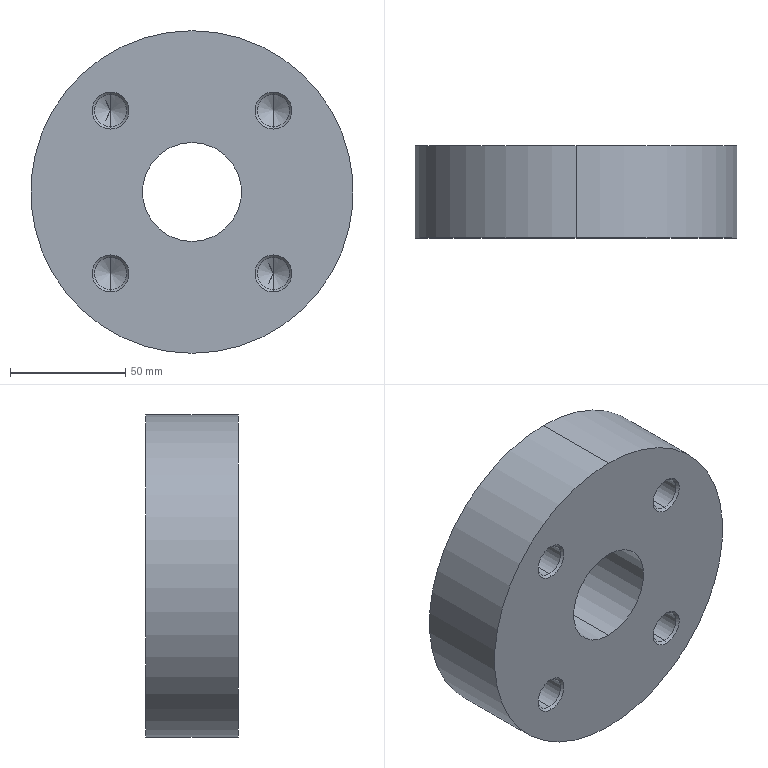Part | SolidWorks | features HoleWzd 2, Extrusion 1 | 1 solid | 54 faces | box 140 x 40 x 140 mm | volume 521515 mm3 | cone 32 | cylinder 20 | plane 2 | commonest cylinder face diameters 14 x16 43 x2 140 x2
STEP:
#1=CARTESIAN_POINT('',(35.355,1.025,-28.355));
#2=VERTEX_POINT('',#1);
#3=CARTESIAN_POINT('',(35.355,1.025,-42.355));
#4=VERTEX_POINT('',#3);
#5=CARTESIAN_POINT('',(35.355,1.025,-35.355));
#6=DIRECTION('',(0.,-1.,0.));
#7=DIRECTION('',(0.,0.,-1.));
#8=AXIS2_PLACEMENT_3D('',#5,#6,#7);
#9=CIRCLE('',#8,7.);
#10=EDGE_CURVE('',#2,#4,#9,.T.);
#11=ORIENTED_EDGE('',*,*,#10,.F.);
#12=CARTESIAN_POINT('',(35.355,0.,-27.33));
#13=VERTEX_POINT('',#12);
#14=CARTESIAN_POINT('',(35.355,0.,-27.33));
#15=DIRECTION('',(0.,-0.7071,0.7071));
#16=VECTOR('',#15,1000.);
#17=LINE('',#14,#16);
#18=EDGE_CURVE('',#2,#13,#17,.T.);
#19=ORIENTED_EDGE('',*,*,#18,.T.);
#20=CARTESIAN_POINT('',(35.355,0.,-43.38));
#21=VERTEX_POINT('',#20);
#22=CARTESIAN_POINT('',(35.355,0.,-35.355));
#23=DIRECTION('',(0.,-1.,0.));
#24=DIRECTION('',(0.,0.,-1.));
#25=AXIS2_PLACEMENT_3D('',#22,#23,#24);
#26=CIRCLE('',#25,8.025);
#27=EDGE_CURVE('',#13,#21,#26,.T.);
#28=ORIENTED_EDGE('',*,*,#27,.T.);
#29=CARTESIAN_POINT('',(35.355,0.,-43.38));
#30=DIRECTION('',(0.,-0.7071,-0.7071));
#31=VECTOR('',#30,1000.);
#32=LINE('',#29,#31);
#33=EDGE_CURVE('',#4,#21,#32,.T.);
#34=ORIENTED_EDGE('',*,*,#33,.F.);
#35=EDGE_LOOP('',(#11,#19,#28,#34));
#36=FACE_OUTER_BOUND('',#35,.T.);
#37=CARTESIAN_POINT('',(35.355,0.,-35.355));
#38=DIRECTION('',(0.,-1.,0.));
#39=DIRECTION('',(0.,0.,-1.));
#40=AXIS2_PLACEMENT_3D('',#37,#38,#39);
#41=CONICAL_SURFACE('',#40,8.025,0.7854);
#42=ADVANCED_FACE('',(#36),#41,.F.);
#43=CARTESIAN_POINT('',(35.355,27.794,-28.355));
#44=VERTEX_POINT('',#43);
#45=CARTESIAN_POINT('',(35.355,27.794,-42.355));
#46=VERTEX_POINT('',#45);
#47=CARTESIAN_POINT('',(35.355,27.794,-35.355));
#48=DIRECTION('',(0.,-1.,0.));
#49=DIRECTION('',(0.,0.,-1.));
#50=AXIS2_PLACEMENT_3D('',#47,#48,#49);
#51=CIRCLE('',#50,7.);
#52=EDGE_CURVE('',#44,#46,#51,.T.);
#53=ORIENTED_EDGE('',*,*,#52,.F.);
#54=CARTESIAN_POINT('',(35.355,0.,-28.355));
#55=DIRECTION('',(0.,-1.,0.));
#56=VECTOR('',#55,1000.);
#57=LINE('',#54,#56);
#58=EDGE_CURVE('',#44,#2,#57,.T.);
#59=ORIENTED_EDGE('',*,*,#58,.T.);
#60=ORIENTED_EDGE('',*,*,#10,.T.);
#61=CARTESIAN_POINT('',(35.355,0.,-42.355));
#62=DIRECTION('',(0.,-1.,0.));
#63=VECTOR('',#62,1000.);
#64=LINE('',#61,#63);
#65=EDGE_CURVE('',#46,#4,#64,.T.);
#66=ORIENTED_EDGE('',*,*,#65,.F.);
#67=EDGE_LOOP('',(#53,#59,#60,#66));
#68=FACE_OUTER_BOUND('',#67,.T.);
#69=CARTESIAN_POINT('',(35.355,0.,-35.355));
#70=DIRECTION('',(0.,-1.,0.));
#71=DIRECTION('',(0.,0.,-1.));
#72=AXIS2_PLACEMENT_3D('',#69,#70,#71);
#73=CYLINDRICAL_SURFACE('',#72,7.);
#74=ADVANCED_FACE('',(#68),#73,.F.);
#75=CARTESIAN_POINT('',(35.355,32.,-35.355));
#76=VERTEX_POINT('',#75);
#77=CARTESIAN_POINT('',(35.355,27.794,-42.355));
#78=DIRECTION('',(0.,-0.515,-0.8572));
#79=VECTOR('',#78,1000.);
#80=LINE('',#77,#79);
#81=EDGE_CURVE('',#76,#46,#80,.T.);
#82=ORIENTED_EDGE('',*,*,#81,.F.);
#83=CARTESIAN_POINT('',(35.355,27.794,-28.355));
#84=DIRECTION('',(0.,-0.515,0.8572));
#85=VECTOR('',#84,1000.);
#86=LINE('',#83,#85);
#87=EDGE_CURVE('',#76,#44,#86,.T.);
#88=ORIENTED_EDGE('',*,*,#87,.T.);
#89=ORIENTED_EDGE('',*,*,#52,.T.);
#90=EDGE_LOOP('',(#82,#88,#89));
#91=FACE_OUTER_BOUND('',#90,.T.);
#92=CARTESIAN_POINT('',(35.355,27.794,-35.355));
#93=DIRECTION('',(0.,-1.,0.));
#94=DIRECTION('',(0.,0.,-1.));
#95=AXIS2_PLACEMENT_3D('',#92,#93,#94);
#96=CONICAL_SURFACE('',#95,7.,1.03);
#97=ADVANCED_FACE('',(#91),#96,.F.);
#98=CARTESIAN_POINT('',(-35.355,1.025,-28.355));
#99=VERTEX_POINT('',#98);
#100=CARTESIAN_POINT('',(-35.355,1.025,-42.355));
#101=VERTEX_POINT('',#100);
#102=CARTESIAN_POINT('',(-35.355,1.025,-35.355));
#103=DIRECTION('',(0.,-1.,0.));
#104=DIRECTION('',(0.,0.,-1.));
#105=AXIS2_PLACEMENT_3D('',#102,#103,#104);
#106=CIRCLE('',#105,7.);
#107=EDGE_CURVE('',#99,#101,#106,.T.);
#108=ORIENTED_EDGE('',*,*,#107,.F.);
#109=CARTESIAN_POINT('',(-35.355,0.,-27.33));
#110=VERTEX_POINT('',#109);
#111=CARTESIAN_POINT('',(-35.355,0.,-27.33));
#112=DIRECTION('',(0.,-0.7071,0.7071));
#113=VECTOR('',#112,1000.);
#114=LINE('',#111,#113);
#115=EDGE_CURVE('',#99,#110,#114,.T.);
#116=ORIENTED_EDGE('',*,*,#115,.T.);
#117=CARTESIAN_POINT('',(-35.355,0.,-43.38));
#118=VERTEX_POINT('',#117);
#119=CARTESIAN_POINT('',(-35.355,0.,-35.355));
#120=DIRECTION('',(0.,-1.,0.));
#121=DIRECTION('',(0.,0.,-1.));
#122=AXIS2_PLACEMENT_3D('',#119,#120,#121);
#123=CIRCLE('',#122,8.025);
#124=EDGE_CURVE('',#110,#118,#123,.T.);
#125=ORIENTED_EDGE('',*,*,#124,.T.);
#126=CARTESIAN_POINT('',(-35.355,0.,-43.38));
#127=DIRECTION('',(0.,-0.7071,-0.7071));
#128=VECTOR('',#127,1000.);
#129=LINE('',#126,#128);
#130=EDGE_CURVE('',#101,#118,#129,.T.);
#131=ORIENTED_EDGE('',*,*,#130,.F.);
#132=EDGE_LOOP('',(#108,#116,#125,#131));
#133=FACE_OUTER_BOUND('',#132,.T.);
#134=CARTESIAN_POINT('',(-35.355,0.,-35.355));
#135=DIRECTION('',(0.,-1.,0.));
#136=DIRECTION('',(0.,0.,-1.));
#137=AXIS2_PLACEMENT_3D('',#134,#135,#136);
#138=CONICAL_SURFACE('',#137,8.025,0.7854);
#139=ADVANCED_FACE('',(#133),#138,.F.);
#140=CARTESIAN_POINT('',(-35.355,27.794,-28.355));
#141=VERTEX_POINT('',#140);
#142=CARTESIAN_POINT('',(-35.355,27.794,-42.355));
#143=VERTEX_POINT('',#142);
#144=CARTESIAN_POINT('',(-35.355,27.794,-35.355));
#145=DIRECTION('',(0.,-1.,0.));
#146=DIRECTION('',(0.,0.,-1.));
#147=AXIS2_PLACEMENT_3D('',#144,#145,#146);
#148=CIRCLE('',#147,7.);
#149=EDGE_CURVE('',#141,#143,#148,.T.);
#150=ORIENTED_EDGE('',*,*,#149,.F.);
#151=CARTESIAN_POINT('',(-35.355,0.,-28.355));
#152=DIRECTION('',(0.,-1.,0.));
#153=VECTOR('',#152,1000.);
#154=LINE('',#151,#153);
#155=EDGE_CURVE('',#141,#99,#154,.T.);
#156=ORIENTED_EDGE('',*,*,#155,.T.);
#157=ORIENTED_EDGE('',*,*,#107,.T.);
#158=CARTESIAN_POINT('',(-35.355,0.,-42.355));
#159=DIRECTION('',(0.,-1.,0.));
#160=VECTOR('',#159,1000.);
#161=LINE('',#158,#160);
#162=EDGE_CURVE('',#143,#101,#161,.T.);
#163=ORIENTED_EDGE('',*,*,#162,.F.);
#164=EDGE_LOOP('',(#150,#156,#157,#163));
#165=FACE_OUTER_BOUND('',#164,.T.);
#166=CARTESIAN_POINT('',(-35.355,0.,-35.355));
#167=DIRECTION('',(0.,-1.,0.));
#168=DIRECTION('',(0.,0.,-1.));
#169=AXIS2_PLACEMENT_3D('',#166,#167,#168);
#170=CYLINDRICAL_SURFACE('',#169,7.);
#171=ADVANCED_FACE('',(#165),#170,.F.);
#172=CARTESIAN_POINT('',(-35.355,32.,-35.355));
#173=VERTEX_POINT('',#172);
#174=CARTESIAN_POINT('',(-35.355,27.794,-42.355));
#175=DIRECTION('',(0.,-0.515,-0.8572));
#176=VECTOR('',#175,1000.);
#177=LINE('',#174,#176);
#178=EDGE_CURVE('',#173,#143,#177,.T.);
#179=ORIENTED_EDGE('',*,*,#178,.F.);
#180=CARTESIAN_POINT('',(-35.355,27.794,-28.355));
#181=DIRECTION('',(0.,-0.515,0.8572));
#182=VECTOR('',#181,1000.);
#183=LINE('',#180,#182);
#184=EDGE_CURVE('',#173,#141,#183,.T.);
#185=ORIENTED_EDGE('',*,*,#184,.T.);
#186=ORIENTED_EDGE('',*,*,#149,.T.);
#187=EDGE_LOOP('',(#179,#185,#186));
#188=FACE_OUTER_BOUND('',#187,.T.);
#189=CARTESIAN_POINT('',(-35.355,27.794,-35.355));
#190=DIRECTION('',(0.,-1.,0.));
#191=DIRECTION('',(0.,0.,-1.));
#192=AXIS2_PLACEMENT_3D('',#189,#190,#191);
#193=CONICAL_SURFACE('',#192,7.,1.03);
#194=ADVANCED_FACE('',(#188),#193,.F.);
#195=CARTESIAN_POINT('',(-35.355,1.025,42.355));
#196=VERTEX_POINT('',#195);
#197=CARTESIAN_POINT('',(-35.355,1.025,28.355));
#198=VERTEX_POINT('',#197);
#199=CARTESIAN_POINT('',(-35.355,1.025,35.355));
#200=DIRECTION('',(0.,-1.,0.));
#201=DIRECTION('',(0.,0.,-1.));
#202=AXIS2_PLACEMENT_3D('',#199,#200,#201);
#203=CIRCLE('',#202,7.);
#204=EDGE_CURVE('',#196,#198,#203,.T.);
#205=ORIENTED_EDGE('',*,*,#204,.F.);
#206=CARTESIAN_POINT('',(-35.355,0.,43.38));
#207=VERTEX_POINT('',#206);
#208=CARTESIAN_POINT('',(-35.355,0.,43.38));
#209=DIRECTION('',(0.,-0.7071,0.7071));
#210=VECTOR('',#209,1000.);
#211=LINE('',#208,#210);
#212=EDGE_CURVE('',#196,#207,#211,.T.);
#213=ORIENTED_EDGE('',*,*,#212,.T.);
#214=CARTESIAN_POINT('',(-35.355,0.,27.33));
#215=VERTEX_POINT('',#214);
#216=CARTESIAN_POINT('',(-35.355,0.,35.355));
#217=DIRECTION('',(0.,-1.,0.));
#218=DIRECTION('',(0.,0.,-1.));
#219=AXIS2_PLACEMENT_3D('',#216,#217,#218);
#220=CIRCLE('',#219,8.025);
#221=EDGE_CURVE('',#207,#215,#220,.T.);
#222=ORIENTED_EDGE('',*,*,#221,.T.);
#223=CARTESIAN_POINT('',(-35.355,0.,27.33));
#224=DIRECTION('',(0.,-0.7071,-0.7071));
#225=VECTOR('',#224,1000.);
#226=LINE('',#223,#225);
#227=EDGE_CURVE('',#198,#215,#226,.T.);
#228=ORIENTED_EDGE('',*,*,#227,.F.);
#229=EDGE_LOOP('',(#205,#213,#222,#228));
#230=FACE_OUTER_BOUND('',#229,.T.);
#231=CARTESIAN_POINT('',(-35.355,0.,35.355));
#232=DIRECTION('',(0.,-1.,0.));
#233=DIRECTION('',(0.,0.,-1.));
#234=AXIS2_PLACEMENT_3D('',#231,#232,#233);
#235=CONICAL_SURFACE('',#234,8.025,0.7854);
#236=ADVANCED_FACE('',(#230),#235,.F.);
#237=CARTESIAN_POINT('',(-35.355,27.794,42.355));
#238=VERTEX_POINT('',#237);
#239=CARTESIAN_POINT('',(-35.355,27.794,28.355));
#240=VERTEX_POINT('',#239);
#241=CARTESIAN_POINT('',(-35.355,27.794,35.355));
#242=DIRECTION('',(0.,-1.,0.));
#243=DIRECTION('',(0.,0.,-1.));
#244=AXIS2_PLACEMENT_3D('',#241,#242,#243);
#245=CIRCLE('',#244,7.);
#246=EDGE_CURVE('',#238,#240,#245,.T.);
#247=ORIENTED_EDGE('',*,*,#246,.F.);
#248=CARTESIAN_POINT('',(-35.355,0.,42.355));
#249=DIRECTION('',(0.,-1.,0.));
#250=VECTOR('',#249,1000.);
#251=LINE('',#248,#250);
#252=EDGE_CURVE('',#238,#196,#251,.T.);
#253=ORIENTED_EDGE('',*,*,#252,.T.);
#254=ORIENTED_EDGE('',*,*,#204,.T.);
#255=CARTESIAN_POINT('',(-35.355,0.,28.355));
#256=DIRECTION('',(0.,-1.,0.));
#257=VECTOR('',#256,1000.);
#258=LINE('',#255,#257);
#259=EDGE_CURVE('',#240,#198,#258,.T.);
#260=ORIENTED_EDGE('',*,*,#259,.F.);
#261=EDGE_LOOP('',(#247,#253,#254,#260));
#262=FACE_OUTER_BOUND('',#261,.T.);
#263=CARTESIAN_POINT('',(-35.355,0.,35.355));
#264=DIRECTION('',(0.,-1.,0.));
#265=DIRECTION('',(0.,0.,-1.));
#266=AXIS2_PLACEMENT_3D('',#263,#264,#265);
#267=CYLINDRICAL_SURFACE('',#266,7.);
#268=ADVANCED_FACE('',(#262),#267,.F.);
#269=CARTESIAN_POINT('',(-35.355,32.,35.355));
#270=VERTEX_POINT('',#269);
#271=CARTESIAN_POINT('',(-35.355,27.794,28.355));
#272=DIRECTION('',(0.,-0.515,-0.8572));
#273=VECTOR('',#272,1000.);
#274=LINE('',#271,#273);
#275=EDGE_CURVE('',#270,#240,#274,.T.);
#276=ORIENTED_EDGE('',*,*,#275,.F.);
#277=CARTESIAN_POINT('',(-35.355,27.794,42.355));
#278=DIRECTION('',(0.,-0.515,0.8572));
#279=VECTOR('',#278,1000.);
#280=LINE('',#277,#279);
#281=EDGE_CURVE('',#270,#238,#280,.T.);
#282=ORIENTED_EDGE('',*,*,#281,.T.);
#283=ORIENTED_EDGE('',*,*,#246,.T.);
#284=EDGE_LOOP('',(#276,#282,#283));
#285=FACE_OUTER_BOUND('',#284,.T.);
#286=CARTESIAN_POINT('',(-35.355,27.794,35.355));
#287=DIRECTION('',(0.,-1.,0.));
#288=DIRECTION('',(0.,0.,-1.));
#289=AXIS2_PLACEMENT_3D('',#286,#287,#288);
#290=CONICAL_SURFACE('',#289,7.,1.03);
#291=ADVANCED_FACE('',(#285),#290,.F.);
#292=CARTESIAN_POINT('',(35.355,1.025,42.355));
#293=VERTEX_POINT('',#292);
#294=CARTESIAN_POINT('',(35.355,1.025,28.355));
#295=VERTEX_POINT('',#294);
#296=CARTESIAN_POINT('',(35.355,1.025,35.355));
#297=DIRECTION('',(0.,-1.,0.));
#298=DIRECTION('',(0.,0.,-1.));
#299=AXIS2_PLACEMENT_3D('',#296,#297,#298);
#300=CIRCLE('',#299,7.);
#301=EDGE_CURVE('',#293,#295,#300,.T.);
#302=ORIENTED_EDGE('',*,*,#301,.F.);
#303=CARTESIAN_POINT('',(35.355,0.,43.38));
#304=VERTEX_POINT('',#303);
#305=CARTESIAN_POINT('',(35.355,0.,43.38));
#306=DIRECTION('',(0.,-0.7071,0.7071));
#307=VECTOR('',#306,1000.);
#308=LINE('',#305,#307);
#309=EDGE_CURVE('',#293,#304,#308,.T.);
#310=ORIENTED_EDGE('',*,*,#309,.T.);
#311=CARTESIAN_POINT('',(35.355,0.,27.33));
#312=VERTEX_POINT('',#311);
#313=CARTESIAN_POINT('',(35.355,0.,35.355));
#314=DIRECTION('',(0.,-1.,0.));
#315=DIRECTION('',(0.,0.,-1.));
#316=AXIS2_PLACEMENT_3D('',#313,#314,#315);
#317=CIRCLE('',#316,8.025);
#318=EDGE_CURVE('',#304,#312,#317,.T.);
#319=ORIENTED_EDGE('',*,*,#318,.T.);
#320=CARTESIAN_POINT('',(35.355,0.,27.33));
#321=DIRECTION('',(0.,-0.7071,-0.7071));
#322=VECTOR('',#321,1000.);
#323=LINE('',#320,#322);
#324=EDGE_CURVE('',#295,#312,#323,.T.);
#325=ORIENTED_EDGE('',*,*,#324,.F.);
#326=EDGE_LOOP('',(#302,#310,#319,#325));
#327=FACE_OUTER_BOUND('',#326,.T.);
#328=CARTESIAN_POINT('',(35.355,0.,35.355));
#329=DIRECTION('',(0.,-1.,0.));
#330=DIRECTION('',(0.,0.,-1.));
#331=AXIS2_PLACEMENT_3D('',#328,#329,#330);
#332=CONICAL_SURFACE('',#331,8.025,0.7854);
#333=ADVANCED_FACE('',(#327),#332,.F.);
#334=CARTESIAN_POINT('',(35.355,27.794,42.355));
#335=VERTEX_POINT('',#334);
#336=CARTESIAN_POINT('',(35.355,27.794,28.355));
#337=VERTEX_POINT('',#336);
#338=CARTESIAN_POINT('',(35.355,27.794,35.355));
#339=DIRECTION('',(0.,-1.,0.));
#340=DIRECTION('',(0.,0.,-1.));
#341=AXIS2_PLACEMENT_3D('',#338,#339,#340);
#342=CIRCLE('',#341,7.);
#343=EDGE_CURVE('',#335,#337,#342,.T.);
#344=ORIENTED_EDGE('',*,*,#343,.F.);
#345=CARTESIAN_POINT('',(35.355,0.,42.355));
#346=DIRECTION('',(0.,-1.,0.));
#347=VECTOR('',#346,1000.);
#348=LINE('',#345,#347);
#349=EDGE_CURVE('',#335,#293,#348,.T.);
#350=ORIENTED_EDGE('',*,*,#349,.T.);
#351=ORIENTED_EDGE('',*,*,#301,.T.);
#352=CARTESIAN_POINT('',(35.355,0.,28.355));
#353=DIRECTION('',(0.,-1.,0.));
#354=VECTOR('',#353,1000.);
#355=LINE('',#352,#354);
#356=EDGE_CURVE('',#337,#295,#355,.T.);
#357=ORIENTED_EDGE('',*,*,#356,.F.);
#358=EDGE_LOOP('',(#344,#350,#351,#357));
#359=FACE_OUTER_BOUND('',#358,.T.);
#360=CARTESIAN_POINT('',(35.355,0.,35.355));
#361=DIRECTION('',(0.,-1.,0.));
#362=DIRECTION('',(0.,0.,-1.));
#363=AXIS2_PLACEMENT_3D('',#360,#361,#362);
#364=CYLINDRICAL_SURFACE('',#363,7.);
#365=ADVANCED_FACE('',(#359),#364,.F.);
#366=CARTESIAN_POINT('',(35.355,32.,35.355));
#367=VERTEX_POINT('',#366);
#368=CARTESIAN_POINT('',(35.355,27.794,28.355));
#369=DIRECTION('',(0.,-0.515,-0.8572));
#370=VECTOR('',#369,1000.);
#371=LINE('',#368,#370);
#372=EDGE_CURVE('',#367,#337,#371,.T.);
#373=ORIENTED_EDGE('',*,*,#372,.F.);
#374=CARTESIAN_POINT('',(35.355,27.794,42.355));
#375=DIRECTION('',(0.,-0.515,0.8572));
#376=VECTOR('',#375,1000.);
#377=LINE('',#374,#376);
#378=EDGE_CURVE('',#367,#335,#377,.T.);
#379=ORIENTED_EDGE('',*,*,#378,.T.);
#380=ORIENTED_EDGE('',*,*,#343,.T.);
#381=EDGE_LOOP('',(#373,#379,#380));
#382=FACE_OUTER_BOUND('',#381,.T.);
#383=CARTESIAN_POINT('',(35.355,27.794,35.355));
#384=DIRECTION('',(0.,-1.,0.));
#385=DIRECTION('',(0.,0.,-1.));
#386=AXIS2_PLACEMENT_3D('',#383,#384,#385);
#387=CONICAL_SURFACE('',#386,7.,1.03);
#388=ADVANCED_FACE('',(#382),#387,.F.);
#389=CARTESIAN_POINT('',(0.,38.975,-57.));
#390=VERTEX_POINT('',#389);
#391=CARTESIAN_POINT('',(0.,38.975,-43.));
#392=VERTEX_POINT('',#391);
#393=CARTESIAN_POINT('',(0.,38.975,-50.));
#394=DIRECTION('',(0.,1.,0.));
#395=DIRECTION('',(0.,0.,1.));
#396=AXIS2_PLACEMENT_3D('',#393,#394,#395);
#397=CIRCLE('',#396,7.);
#398=EDGE_CURVE('',#390,#392,#397,.T.);
#399=ORIENTED_EDGE('',*,*,#398,.F.);
#400=CARTESIAN_POINT('',(0.,40.,-58.025));
#401=VERTEX_POINT('',#400);
#402=CARTESIAN_POINT('',(0.,40.,-58.025));
#403=DIRECTION('',(0.,0.7071,-0.7071));
#404=VECTOR('',#403,1000.);
#405=LINE('',#402,#404);
#406=EDGE_CURVE('',#390,#401,#405,.T.);
#407=ORIENTED_EDGE('',*,*,#406,.T.);
#408=CARTESIAN_POINT('',(0.,40.,-41.975));
#409=VERTEX_POINT('',#408);
#410=CARTESIAN_POINT('',(0.,40.,-50.));
#411=DIRECTION('',(0.,1.,0.));
#412=DIRECTION('',(0.,0.,1.));
#413=AXIS2_PLACEMENT_3D('',#410,#411,#412);
#414=CIRCLE('',#413,8.025);
#415=EDGE_CURVE('',#401,#409,#414,.T.);
#416=ORIENTED_EDGE('',*,*,#415,.T.);
#417=CARTESIAN_POINT('',(0.,40.,-41.975));
#418=DIRECTION('',(0.,0.7071,0.7071));
#419=VECTOR('',#418,1000.);
#420=LINE('',#417,#419);
#421=EDGE_CURVE('',#392,#409,#420,.T.);
#422=ORIENTED_EDGE('',*,*,#421,.F.);
#423=EDGE_LOOP('',(#399,#407,#416,#422));
#424=FACE_OUTER_BOUND('',#423,.T.);
#425=CARTESIAN_POINT('',(0.,40.,-50.));
#426=DIRECTION('',(0.,1.,0.));
#427=DIRECTION('',(0.,0.,1.));
#428=AXIS2_PLACEMENT_3D('',#425,#426,#427);
#429=CONICAL_SURFACE('',#428,8.025,0.7854);
#430=ADVANCED_FACE('',(#424),#429,.F.);
#431=CARTESIAN_POINT('',(0.,12.206,-57.));
#432=VERTEX_POINT('',#431);
#433=CARTESIAN_POINT('',(0.,12.206,-43.));
#434=VERTEX_POINT('',#433);
#435=CARTESIAN_POINT('',(0.,12.206,-50.));
#436=DIRECTION('',(0.,1.,0.));
#437=DIRECTION('',(0.,0.,1.));
#438=AXIS2_PLACEMENT_3D('',#435,#436,#437);
#439=CIRCLE('',#438,7.);
#440=EDGE_CURVE('',#432,#434,#439,.T.);
#441=ORIENTED_EDGE('',*,*,#440,.F.);
#442=CARTESIAN_POINT('',(0.,40.,-57.));
#443=DIRECTION('',(0.,1.,0.));
#444=VECTOR('',#443,1000.);
#445=LINE('',#442,#444);
#446=EDGE_CURVE('',#432,#390,#445,.T.);
#447=ORIENTED_EDGE('',*,*,#446,.T.);
#448=ORIENTED_EDGE('',*,*,#398,.T.);
#449=CARTESIAN_POINT('',(0.,40.,-43.));
#450=DIRECTION('',(0.,1.,0.));
#451=VECTOR('',#450,1000.);
#452=LINE('',#449,#451);
#453=EDGE_CURVE('',#434,#392,#452,.T.);
#454=ORIENTED_EDGE('',*,*,#453,.F.);
#455=EDGE_LOOP('',(#441,#447,#448,#454));
#456=FACE_OUTER_BOUND('',#455,.T.);
#457=CARTESIAN_POINT('',(0.,40.,-50.));
#458=DIRECTION('',(0.,1.,0.));
#459=DIRECTION('',(0.,0.,1.));
#460=AXIS2_PLACEMENT_3D('',#457,#458,#459);
#461=CYLINDRICAL_SURFACE('',#460,7.);
#462=ADVANCED_FACE('',(#456),#461,.F.);
#463=CARTESIAN_POINT('',(0.,8.,-50.));
#464=VERTEX_POINT('',#463);
#465=CARTESIAN_POINT('',(0.,12.206,-43.));
#466=DIRECTION('',(0.,0.515,0.8572));
#467=VECTOR('',#466,1000.);
#468=LINE('',#465,#467);
#469=EDGE_CURVE('',#464,#434,#468,.T.);
#470=ORIENTED_EDGE('',*,*,#469,.F.);
#471=CARTESIAN_POINT('',(0.,12.206,-57.));
#472=DIRECTION('',(0.,0.515,-0.8572));
#473=VECTOR('',#472,1000.);
#474=LINE('',#471,#473);
#475=EDGE_CURVE('',#464,#432,#474,.T.);
#476=ORIENTED_EDGE('',*,*,#475,.T.);
#477=ORIENTED_EDGE('',*,*,#440,.T.);
#478=EDGE_LOOP('',(#470,#476,#477));
#479=FACE_OUTER_BOUND('',#478,.T.);
#480=CARTESIAN_POINT('',(0.,12.206,-50.));
#481=DIRECTION('',(0.,1.,0.));
#482=DIRECTION('',(0.,0.,1.));
#483=AXIS2_PLACEMENT_3D('',#480,#481,#482);
#484=CONICAL_SURFACE('',#483,7.,1.03);
#485=ADVANCED_FACE('',(#479),#484,.F.);
#486=CARTESIAN_POINT('',(50.,38.975,-7.));
#487=VERTEX_POINT('',#486);
#488=CARTESIAN_POINT('',(50.,38.975,7.));
#489=VERTEX_POINT('',#488);
#490=CARTESIAN_POINT('',(50.,38.975,0.));
#491=DIRECTION('',(0.,1.,0.));
#492=DIRECTION('',(0.,0.,1.));
#493=AXIS2_PLACEMENT_3D('',#490,#491,#492);
#494=CIRCLE('',#493,7.);
#495=EDGE_CURVE('',#487,#489,#494,.T.);
#496=ORIENTED_EDGE('',*,*,#495,.F.);
#497=CARTESIAN_POINT('',(50.,40.,-8.025));
#498=VERTEX_POINT('',#497);
#499=CARTESIAN_POINT('',(50.,40.,-8.025));
#500=DIRECTION('',(0.,0.7071,-0.7071));
#501=VECTOR('',#500,1000.);
#502=LINE('',#499,#501);
#503=EDGE_CURVE('',#487,#498,#502,.T.);
#504=ORIENTED_EDGE('',*,*,#503,.T.);
#505=CARTESIAN_POINT('',(50.,40.,8.025));
#506=VERTEX_POINT('',#505);
#507=CARTESIAN_POINT('',(50.,40.,0.));
#508=DIRECTION('',(0.,1.,0.));
#509=DIRECTION('',(0.,0.,1.));
#510=AXIS2_PLACEMENT_3D('',#507,#508,#509);
#511=CIRCLE('',#510,8.025);
#512=EDGE_CURVE('',#498,#506,#511,.T.);
#513=ORIENTED_EDGE('',*,*,#512,.T.);
#514=CARTESIAN_POINT('',(50.,40.,8.025));
#515=DIRECTION('',(0.,0.7071,0.7071));
#516=VECTOR('',#515,1000.);
#517=LINE('',#514,#516);
#518=EDGE_CURVE('',#489,#506,#517,.T.);
#519=ORIENTED_EDGE('',*,*,#518,.F.);
#520=EDGE_LOOP('',(#496,#504,#513,#519));
#521=FACE_OUTER_BOUND('',#520,.T.);
#522=CARTESIAN_POINT('',(50.,40.,0.));
#523=DIRECTION('',(0.,1.,0.));
#524=DIRECTION('',(0.,0.,1.));
#525=AXIS2_PLACEMENT_3D('',#522,#523,#524);
#526=CONICAL_SURFACE('',#525,8.025,0.7854);
#527=ADVANCED_FACE('',(#521),#526,.F.);
#528=CARTESIAN_POINT('',(50.,12.206,-7.));
#529=VERTEX_POINT('',#528);
#530=CARTESIAN_POINT('',(50.,12.206,7.));
#531=VERTEX_POINT('',#530);
#532=CARTESIAN_POINT('',(50.,12.206,0.));
#533=DIRECTION('',(0.,1.,0.));
#534=DIRECTION('',(0.,0.,1.));
#535=AXIS2_PLACEMENT_3D('',#532,#533,#534);
#536=CIRCLE('',#535,7.);
#537=EDGE_CURVE('',#529,#531,#536,.T.);
#538=ORIENTED_EDGE('',*,*,#537,.F.);
#539=CARTESIAN_POINT('',(50.,40.,-7.));
#540=DIRECTION('',(0.,1.,0.));
#541=VECTOR('',#540,1000.);
#542=LINE('',#539,#541);
#543=EDGE_CURVE('',#529,#487,#542,.T.);
#544=ORIENTED_EDGE('',*,*,#543,.T.);
#545=ORIENTED_EDGE('',*,*,#495,.T.);
#546=CARTESIAN_POINT('',(50.,40.,7.));
#547=DIRECTION('',(0.,1.,0.));
#548=VECTOR('',#547,1000.);
#549=LINE('',#546,#548);
#550=EDGE_CURVE('',#531,#489,#549,.T.);
#551=ORIENTED_EDGE('',*,*,#550,.F.);
#552=EDGE_LOOP('',(#538,#544,#545,#551));
#553=FACE_OUTER_BOUND('',#552,.T.);
#554=CARTESIAN_POINT('',(50.,40.,0.));
#555=DIRECTION('',(0.,1.,0.));
#556=DIRECTION('',(0.,0.,1.));
#557=AXIS2_PLACEMENT_3D('',#554,#555,#556);
#558=CYLINDRICAL_SURFACE('',#557,7.);
#559=ADVANCED_FACE('',(#553),#558,.F.);
#560=CARTESIAN_POINT('',(50.,8.,0.));
#561=VERTEX_POINT('',#560);
#562=CARTESIAN_POINT('',(50.,12.206,7.));
#563=DIRECTION('',(0.,0.515,0.8572));
#564=VECTOR('',#563,1000.);
#565=LINE('',#562,#564);
#566=EDGE_CURVE('',#561,#531,#565,.T.);
#567=ORIENTED_EDGE('',*,*,#566,.F.);
#568=CARTESIAN_POINT('',(50.,12.206,-7.));
#569=DIRECTION('',(0.,0.515,-0.8572));
#570=VECTOR('',#569,1000.);
#571=LINE('',#568,#570);
#572=EDGE_CURVE('',#561,#529,#571,.T.);
#573=ORIENTED_EDGE('',*,*,#572,.T.);
#574=ORIENTED_EDGE('',*,*,#537,.T.);
#575=EDGE_LOOP('',(#567,#573,#574));
#576=FACE_OUTER_BOUND('',#575,.T.);
#577=CARTESIAN_POINT('',(50.,12.206,0.));
#578=DIRECTION('',(0.,1.,0.));
#579=DIRECTION('',(0.,0.,1.));
#580=AXIS2_PLACEMENT_3D('',#577,#578,#579);
#581=CONICAL_SURFACE('',#580,7.,1.03);
#582=ADVANCED_FACE('',(#576),#581,.F.);
#583=CARTESIAN_POINT('',(0.,38.975,43.));
#584=VERTEX_POINT('',#583);
#585=CARTESIAN_POINT('',(0.,38.975,57.));
#586=VERTEX_POINT('',#585);
#587=CARTESIAN_POINT('',(0.,38.975,50.));
#588=DIRECTION('',(0.,1.,0.));
#589=DIRECTION('',(0.,0.,1.));
#590=AXIS2_PLACEMENT_3D('',#587,#588,#589);
#591=CIRCLE('',#590,7.);
#592=EDGE_CURVE('',#584,#586,#591,.T.);
#593=ORIENTED_EDGE('',*,*,#592,.F.);
#594=CARTESIAN_POINT('',(0.,40.,41.975));
#595=VERTEX_POINT('',#594);
#596=CARTESIAN_POINT('',(0.,40.,41.975));
#597=DIRECTION('',(0.,0.7071,-0.7071));
#598=VECTOR('',#597,1000.);
#599=LINE('',#596,#598);
#600=EDGE_CURVE('',#584,#595,#599,.T.);
#601=ORIENTED_EDGE('',*,*,#600,.T.);
#602=CARTESIAN_POINT('',(0.,40.,58.025));
#603=VERTEX_POINT('',#602);
#604=CARTESIAN_POINT('',(0.,40.,50.));
#605=DIRECTION('',(0.,1.,0.));
#606=DIRECTION('',(0.,0.,1.));
#607=AXIS2_PLACEMENT_3D('',#604,#605,#606);
#608=CIRCLE('',#607,8.025);
#609=EDGE_CURVE('',#595,#603,#608,.T.);
#610=ORIENTED_EDGE('',*,*,#609,.T.);
#611=CARTESIAN_POINT('',(0.,40.,58.025));
#612=DIRECTION('',(0.,0.7071,0.7071));
#613=VECTOR('',#612,1000.);
#614=LINE('',#611,#613);
#615=EDGE_CURVE('',#586,#603,#614,.T.);
#616=ORIENTED_EDGE('',*,*,#615,.F.);
#617=EDGE_LOOP('',(#593,#601,#610,#616));
#618=FACE_OUTER_BOUND('',#617,.T.);
#619=CARTESIAN_POINT('',(0.,40.,50.));
#620=DIRECTION('',(0.,1.,0.));
#621=DIRECTION('',(0.,0.,1.));
#622=AXIS2_PLACEMENT_3D('',#619,#620,#621);
#623=CONICAL_SURFACE('',#622,8.025,0.7854);
#624=ADVANCED_FACE('',(#618),#623,.F.);
#625=CARTESIAN_POINT('',(0.,12.206,43.));
#626=VERTEX_POINT('',#625);
#627=CARTESIAN_POINT('',(0.,12.206,57.));
#628=VERTEX_POINT('',#627);
#629=CARTESIAN_POINT('',(0.,12.206,50.));
#630=DIRECTION('',(0.,1.,0.));
#631=DIRECTION('',(0.,0.,1.));
#632=AXIS2_PLACEMENT_3D('',#629,#630,#631);
#633=CIRCLE('',#632,7.);
#634=EDGE_CURVE('',#626,#628,#633,.T.);
#635=ORIENTED_EDGE('',*,*,#634,.F.);
#636=CARTESIAN_POINT('',(0.,40.,43.));
#637=DIRECTION('',(0.,1.,0.));
#638=VECTOR('',#637,1000.);
#639=LINE('',#636,#638);
#640=EDGE_CURVE('',#626,#584,#639,.T.);
#641=ORIENTED_EDGE('',*,*,#640,.T.);
#642=ORIENTED_EDGE('',*,*,#592,.T.);
#643=CARTESIAN_POINT('',(0.,40.,57.));
#644=DIRECTION('',(0.,1.,0.));
#645=VECTOR('',#644,1000.);
#646=LINE('',#643,#645);
#647=EDGE_CURVE('',#628,#586,#646,.T.);
#648=ORIENTED_EDGE('',*,*,#647,.F.);
#649=EDGE_LOOP('',(#635,#641,#642,#648));
#650=FACE_OUTER_BOUND('',#649,.T.);
#651=CARTESIAN_POINT('',(0.,40.,50.));
#652=DIRECTION('',(0.,1.,0.));
#653=DIRECTION('',(0.,0.,1.));
#654=AXIS2_PLACEMENT_3D('',#651,#652,#653);
#655=CYLINDRICAL_SURFACE('',#654,7.);
#656=ADVANCED_FACE('',(#650),#655,.F.);
#657=CARTESIAN_POINT('',(0.,8.,50.));
#658=VERTEX_POINT('',#657);
#659=CARTESIAN_POINT('',(0.,12.206,57.));
#660=DIRECTION('',(0.,0.515,0.8572));
#661=VECTOR('',#660,1000.);
#662=LINE('',#659,#661);
#663=EDGE_CURVE('',#658,#628,#662,.T.);
#664=ORIENTED_EDGE('',*,*,#663,.F.);
#665=CARTESIAN_POINT('',(0.,12.206,43.));
#666=DIRECTION('',(0.,0.515,-0.8572));
#667=VECTOR('',#666,1000.);
#668=LINE('',#665,#667);
#669=EDGE_CURVE('',#658,#626,#668,.T.);
#670=ORIENTED_EDGE('',*,*,#669,.T.);
#671=ORIENTED_EDGE('',*,*,#634,.T.);
#672=EDGE_LOOP('',(#664,#670,#671));
#673=FACE_OUTER_BOUND('',#672,.T.);
#674=CARTESIAN_POINT('',(0.,12.206,50.));
#675=DIRECTION('',(0.,1.,0.));
#676=DIRECTION('',(0.,0.,1.));
#677=AXIS2_PLACEMENT_3D('',#674,#675,#676);
#678=CONICAL_SURFACE('',#677,7.,1.03);
#679=ADVANCED_FACE('',(#673),#678,.F.);
#680=CARTESIAN_POINT('',(-50.,38.975,-7.));
#681=VERTEX_POINT('',#680);
#682=CARTESIAN_POINT('',(-50.,38.975,7.));
#683=VERTEX_POINT('',#682);
#684=CARTESIAN_POINT('',(-50.,38.975,0.));
#685=DIRECTION('',(0.,1.,0.));
#686=DIRECTION('',(0.,0.,1.));
#687=AXIS2_PLACEMENT_3D('',#684,#685,#686);
#688=CIRCLE('',#687,7.);
#689=EDGE_CURVE('',#681,#683,#688,.T.);
#690=ORIENTED_EDGE('',*,*,#689,.F.);
#691=CARTESIAN_POINT('',(-50.,40.,-8.025));
#692=VERTEX_POINT('',#691);
#693=CARTESIAN_POINT('',(-50.,40.,-8.025));
#694=DIRECTION('',(0.,0.7071,-0.7071));
#695=VECTOR('',#694,1000.);
#696=LINE('',#693,#695);
#697=EDGE_CURVE('',#681,#692,#696,.T.);
#698=ORIENTED_EDGE('',*,*,#697,.T.);
#699=CARTESIAN_POINT('',(-50.,40.,8.025));
#700=VERTEX_POINT('',#699);
#701=CARTESIAN_POINT('',(-50.,40.,0.));
#702=DIRECTION('',(0.,1.,0.));
#703=DIRECTION('',(0.,0.,1.));
#704=AXIS2_PLACEMENT_3D('',#701,#702,#703);
#705=CIRCLE('',#704,8.025);
#706=EDGE_CURVE('',#692,#700,#705,.T.);
#707=ORIENTED_EDGE('',*,*,#706,.T.);
#708=CARTESIAN_POINT('',(-50.,40.,8.025));
#709=DIRECTION('',(0.,0.7071,0.7071));
#710=VECTOR('',#709,1000.);
#711=LINE('',#708,#710);
#712=EDGE_CURVE('',#683,#700,#711,.T.);
#713=ORIENTED_EDGE('',*,*,#712,.F.);
#714=EDGE_LOOP('',(#690,#698,#707,#713));
#715=FACE_OUTER_BOUND('',#714,.T.);
#716=CARTESIAN_POINT('',(-50.,40.,0.));
#717=DIRECTION('',(0.,1.,0.));
#718=DIRECTION('',(0.,0.,1.));
#719=AXIS2_PLACEMENT_3D('',#716,#717,#718);
#720=CONICAL_SURFACE('',#719,8.025,0.7854);
#721=ADVANCED_FACE('',(#715),#720,.F.);
#722=CARTESIAN_POINT('',(-50.,12.206,-7.));
#723=VERTEX_POINT('',#722);
#724=CARTESIAN_POINT('',(-50.,12.206,7.));
#725=VERTEX_POINT('',#724);
#726=CARTESIAN_POINT('',(-50.,12.206,0.));
#727=DIRECTION('',(0.,1.,0.));
#728=DIRECTION('',(0.,0.,1.));
#729=AXIS2_PLACEMENT_3D('',#726,#727,#728);
#730=CIRCLE('',#729,7.);
#731=EDGE_CURVE('',#723,#725,#730,.T.);
#732=ORIENTED_EDGE('',*,*,#731,.F.);
#733=CARTESIAN_POINT('',(-50.,40.,-7.));
#734=DIRECTION('',(0.,1.,0.));
#735=VECTOR('',#734,1000.);
#736=LINE('',#733,#735);
#737=EDGE_CURVE('',#723,#681,#736,.T.);
#738=ORIENTED_EDGE('',*,*,#737,.T.);
#739=ORIENTED_EDGE('',*,*,#689,.T.);
#740=CARTESIAN_POINT('',(-50.,40.,7.));
#741=DIRECTION('',(0.,1.,0.));
#742=VECTOR('',#741,1000.);
#743=LINE('',#740,#742);
#744=EDGE_CURVE('',#725,#683,#743,.T.);
#745=ORIENTED_EDGE('',*,*,#744,.F.);
#746=EDGE_LOOP('',(#732,#738,#739,#745));
#747=FACE_OUTER_BOUND('',#746,.T.);
#748=CARTESIAN_POINT('',(-50.,40.,0.));
#749=DIRECTION('',(0.,1.,0.));
#750=DIRECTION('',(0.,0.,1.));
#751=AXIS2_PLACEMENT_3D('',#748,#749,#750);
#752=CYLINDRICAL_SURFACE('',#751,7.);
#753=ADVANCED_FACE('',(#747),#752,.F.);
#754=CARTESIAN_POINT('',(-50.,8.,0.));
#755=VERTEX_POINT('',#754);
#756=CARTESIAN_POINT('',(-50.,12.206,7.));
#757=DIRECTION('',(0.,0.515,0.8572));
#758=VECTOR('',#757,1000.);
#759=LINE('',#756,#758);
#760=EDGE_CURVE('',#755,#725,#759,.T.);
#761=ORIENTED_EDGE('',*,*,#760,.F.);
#762=CARTESIAN_POINT('',(-50.,12.206,-7.));
#763=DIRECTION('',(0.,0.515,-0.8572));
#764=VECTOR('',#763,1000.);
#765=LINE('',#762,#764);
#766=EDGE_CURVE('',#755,#723,#765,.T.);
#767=ORIENTED_EDGE('',*,*,#766,.T.);
#768=ORIENTED_EDGE('',*,*,#731,.T.);
#769=EDGE_LOOP('',(#761,#767,#768));
#770=FACE_OUTER_BOUND('',#769,.T.);
#771=CARTESIAN_POINT('',(-50.,12.206,0.));
#772=DIRECTION('',(0.,1.,0.));
#773=DIRECTION('',(0.,0.,1.));
#774=AXIS2_PLACEMENT_3D('',#771,#772,#773);
#775=CONICAL_SURFACE('',#774,7.,1.03);
#776=ADVANCED_FACE('',(#770),#775,.F.);
#777=CARTESIAN_POINT('',(0.,40.,-21.5));
#778=VERTEX_POINT('',#777);
#779=CARTESIAN_POINT('',(0.,40.,21.5));
#780=VERTEX_POINT('',#779);
#781=CARTESIAN_POINT('',(0.,40.,0.));
#782=DIRECTION('',(0.,1.,0.));
#783=DIRECTION('',(0.,0.,1.));
#784=AXIS2_PLACEMENT_3D('',#781,#782,#783);
#785=CIRCLE('',#784,21.5);
#786=EDGE_CURVE('',#778,#780,#785,.T.);
#787=ORIENTED_EDGE('',*,*,#786,.T.);
#788=CARTESIAN_POINT('',(0.,0.,21.5));
#789=VERTEX_POINT('',#788);
#790=CARTESIAN_POINT('',(0.,40.,21.5));
#791=DIRECTION('',(0.,-1.,0.));
#792=VECTOR('',#791,1000.);
#793=LINE('',#790,#792);
#794=EDGE_CURVE('',#780,#789,#793,.T.);
#795=ORIENTED_EDGE('',*,*,#794,.T.);
#796=CARTESIAN_POINT('',(0.,0.,-21.5));
#797=VERTEX_POINT('',#796);
#798=CARTESIAN_POINT('',(0.,0.,0.));
#799=DIRECTION('',(0.,1.,0.));
#800=DIRECTION('',(0.,0.,1.));
#801=AXIS2_PLACEMENT_3D('',#798,#799,#800);
#802=CIRCLE('',#801,21.5);
#803=EDGE_CURVE('',#797,#789,#802,.T.);
#804=ORIENTED_EDGE('',*,*,#803,.F.);
#805=CARTESIAN_POINT('',(0.,40.,-21.5));
#806=DIRECTION('',(0.,-1.,0.));
#807=VECTOR('',#806,1000.);
#808=LINE('',#805,#807);
#809=EDGE_CURVE('',#778,#797,#808,.T.);
#810=ORIENTED_EDGE('',*,*,#809,.F.);
#811=EDGE_LOOP('',(#787,#795,#804,#810));
#812=FACE_OUTER_BOUND('',#811,.T.);
#813=CARTESIAN_POINT('',(0.,40.,0.));
#814=DIRECTION('',(0.,-1.,0.));
#815=DIRECTION('',(0.,0.,-1.));
#816=AXIS2_PLACEMENT_3D('',#813,#814,#815);
#817=CYLINDRICAL_SURFACE('',#816,21.5);
#818=ADVANCED_FACE('',(#812),#817,.F.);
#819=CARTESIAN_POINT('',(0.,40.,70.));
#820=VERTEX_POINT('',#819);
#821=CARTESIAN_POINT('',(0.,40.,-70.));
#822=VERTEX_POINT('',#821);
#823=CARTESIAN_POINT('',(0.,40.,0.));
#824=DIRECTION('',(0.,1.,0.));
#825=DIRECTION('',(0.,0.,1.));
#826=AXIS2_PLACEMENT_3D('',#823,#824,#825);
#827=CIRCLE('',#826,70.);
#828=EDGE_CURVE('',#820,#822,#827,.T.);
#829=ORIENTED_EDGE('',*,*,#828,.F.);
#830=CARTESIAN_POINT('',(0.,0.,70.));
#831=VERTEX_POINT('',#830);
#832=CARTESIAN_POINT('',(0.,40.,70.));
#833=DIRECTION('',(0.,-1.,0.));
#834=VECTOR('',#833,1000.);
#835=LINE('',#832,#834);
#836=EDGE_CURVE('',#820,#831,#835,.T.);
#837=ORIENTED_EDGE('',*,*,#836,.T.);
#838=CARTESIAN_POINT('',(0.,0.,-70.));
#839=VERTEX_POINT('',#838);
#840=CARTESIAN_POINT('',(0.,0.,0.));
#841=DIRECTION('',(0.,1.,0.));
#842=DIRECTION('',(0.,0.,1.));
#843=AXIS2_PLACEMENT_3D('',#840,#841,#842);
#844=CIRCLE('',#843,70.);
#845=EDGE_CURVE('',#831,#839,#844,.T.);
#846=ORIENTED_EDGE('',*,*,#845,.T.);
#847=CARTESIAN_POINT('',(0.,40.,-70.));
#848=DIRECTION('',(0.,-1.,0.));
#849=VECTOR('',#848,1000.);
#850=LINE('',#847,#849);
#851=EDGE_CURVE('',#822,#839,#850,.T.);
#852=ORIENTED_EDGE('',*,*,#851,.F.);
#853=EDGE_LOOP('',(#829,#837,#846,#852));
#854=FACE_OUTER_BOUND('',#853,.T.);
#855=CARTESIAN_POINT('',(0.,40.,0.));
#856=DIRECTION('',(0.,-1.,0.));
#857=DIRECTION('',(0.,0.,-1.));
#858=AXIS2_PLACEMENT_3D('',#855,#856,#857);
#859=CYLINDRICAL_SURFACE('',#858,70.);
#860=ADVANCED_FACE('',(#854),#859,.T.);
#861=CARTESIAN_POINT('',(0.,40.,-50.));
#862=DIRECTION('',(0.,1.,0.));
#863=DIRECTION('',(0.,0.,1.));
#864=AXIS2_PLACEMENT_3D('',#861,#862,#863);
#865=CIRCLE('',#864,8.025);
#866=EDGE_CURVE('',#409,#401,#865,.T.);
#867=ORIENTED_EDGE('',*,*,#866,.F.);
#868=ORIENTED_EDGE('',*,*,#415,.F.);
#869=EDGE_LOOP('',(#867,#868));
#870=FACE_BOUND('',#869,.T.);
#871=CARTESIAN_POINT('',(50.,40.,0.));
#872=DIRECTION('',(0.,1.,0.));
#873=DIRECTION('',(0.,0.,1.));
#874=AXIS2_PLACEMENT_3D('',#871,#872,#873);
#875=CIRCLE('',#874,8.025);
#876=EDGE_CURVE('',#506,#498,#875,.T.);
#877=ORIENTED_EDGE('',*,*,#876,.F.);
#878=ORIENTED_EDGE('',*,*,#512,.F.);
#879=EDGE_LOOP('',(#877,#878));
#880=FACE_BOUND('',#879,.T.);
#881=CARTESIAN_POINT('',(0.,40.,50.));
#882=DIRECTION('',(0.,1.,0.));
#883=DIRECTION('',(0.,0.,1.));
#884=AXIS2_PLACEMENT_3D('',#881,#882,#883);
#885=CIRCLE('',#884,8.025);
#886=EDGE_CURVE('',#603,#595,#885,.T.);
#887=ORIENTED_EDGE('',*,*,#886,.F.);
#888=ORIENTED_EDGE('',*,*,#609,.F.);
#889=EDGE_LOOP('',(#887,#888));
#890=FACE_BOUND('',#889,.T.);
#891=CARTESIAN_POINT('',(-50.,40.,0.));
#892=DIRECTION('',(0.,1.,0.));
#893=DIRECTION('',(0.,0.,1.));
#894=AXIS2_PLACEMENT_3D('',#891,#892,#893);
#895=CIRCLE('',#894,8.025);
#896=EDGE_CURVE('',#700,#692,#895,.T.);
#897=ORIENTED_EDGE('',*,*,#896,.F.);
#898=ORIENTED_EDGE('',*,*,#706,.F.);
#899=EDGE_LOOP('',(#897,#898));
#900=FACE_BOUND('',#899,.T.);
#901=CARTESIAN_POINT('',(0.,40.,0.));
#902=DIRECTION('',(0.,1.,0.));
#903=DIRECTION('',(0.,0.,1.));
#904=AXIS2_PLACEMENT_3D('',#901,#902,#903);
#905=CIRCLE('',#904,70.);
#906=EDGE_CURVE('',#822,#820,#905,.T.);
#907=ORIENTED_EDGE('',*,*,#906,.T.);
#908=ORIENTED_EDGE('',*,*,#828,.T.);
#909=EDGE_LOOP('',(#907,#908));
#910=FACE_OUTER_BOUND('',#909,.T.);
#911=ORIENTED_EDGE('',*,*,#786,.F.);
#912=CARTESIAN_POINT('',(0.,40.,0.));
#913=DIRECTION('',(0.,1.,0.));
#914=DIRECTION('',(0.,0.,1.));
#915=AXIS2_PLACEMENT_3D('',#912,#913,#914);
#916=CIRCLE('',#915,21.5);
#917=EDGE_CURVE('',#780,#778,#916,.T.);
#918=ORIENTED_EDGE('',*,*,#917,.F.);
#919=EDGE_LOOP('',(#911,#918));
#920=FACE_BOUND('',#919,.T.);
#921=CARTESIAN_POINT('',(0.,40.,0.));
#922=DIRECTION('',(0.,1.,0.));
#923=DIRECTION('',(0.,0.,1.));
#924=AXIS2_PLACEMENT_3D('',#921,#922,#923);
#925=PLANE('',#924);
#926=ADVANCED_FACE('',(#870,#880,#890,#900,#910,#920),#925,.T.);
#927=CARTESIAN_POINT('',(35.355,0.,-35.355));
#928=DIRECTION('',(0.,-1.,0.));
#929=DIRECTION('',(0.,0.,-1.));
#930=AXIS2_PLACEMENT_3D('',#927,#928,#929);
#931=CIRCLE('',#930,8.025);
#932=EDGE_CURVE('',#21,#13,#931,.T.);
#933=ORIENTED_EDGE('',*,*,#932,.F.);
#934=ORIENTED_EDGE('',*,*,#27,.F.);
#935=EDGE_LOOP('',(#933,#934));
#936=FACE_BOUND('',#935,.T.);
#937=CARTESIAN_POINT('',(-35.355,0.,-35.355));
#938=DIRECTION('',(0.,-1.,0.));
#939=DIRECTION('',(0.,0.,-1.));
#940=AXIS2_PLACEMENT_3D('',#937,#938,#939);
#941=CIRCLE('',#940,8.025);
#942=EDGE_CURVE('',#118,#110,#941,.T.);
#943=ORIENTED_EDGE('',*,*,#942,.F.);
#944=ORIENTED_EDGE('',*,*,#124,.F.);
#945=EDGE_LOOP('',(#943,#944));
#946=FACE_BOUND('',#945,.T.);
#947=CARTESIAN_POINT('',(-35.355,0.,35.355));
#948=DIRECTION('',(0.,-1.,0.));
#949=DIRECTION('',(0.,0.,-1.));
#950=AXIS2_PLACEMENT_3D('',#947,#948,#949);
#951=CIRCLE('',#950,8.025);
#952=EDGE_CURVE('',#215,#207,#951,.T.);
#953=ORIENTED_EDGE('',*,*,#952,.F.);
#954=ORIENTED_EDGE('',*,*,#221,.F.);
#955=EDGE_LOOP('',(#953,#954));
#956=FACE_BOUND('',#955,.T.);
#957=CARTESIAN_POINT('',(35.355,0.,35.355));
#958=DIRECTION('',(0.,-1.,0.));
#959=DIRECTION('',(0.,0.,-1.));
#960=AXIS2_PLACEMENT_3D('',#957,#958,#959);
#961=CIRCLE('',#960,8.025);
#962=EDGE_CURVE('',#312,#304,#961,.T.);
#963=ORIENTED_EDGE('',*,*,#962,.F.);
#964=ORIENTED_EDGE('',*,*,#318,.F.);
#965=EDGE_LOOP('',(#963,#964));
#966=FACE_BOUND('',#965,.T.);
#967=CARTESIAN_POINT('',(0.,0.,0.));
#968=DIRECTION('',(0.,1.,0.));
#969=DIRECTION('',(0.,0.,1.));
#970=AXIS2_PLACEMENT_3D('',#967,#968,#969);
#971=CIRCLE('',#970,70.);
#972=EDGE_CURVE('',#839,#831,#971,.T.);
#973=ORIENTED_EDGE('',*,*,#972,.F.);
#974=ORIENTED_EDGE('',*,*,#845,.F.);
#975=EDGE_LOOP('',(#973,#974));
#976=FACE_OUTER_BOUND('',#975,.T.);
#977=ORIENTED_EDGE('',*,*,#803,.T.);
#978=CARTESIAN_POINT('',(0.,0.,0.));
#979=DIRECTION('',(0.,1.,0.));
#980=DIRECTION('',(0.,0.,1.));
#981=AXIS2_PLACEMENT_3D('',#978,#979,#980);
#982=CIRCLE('',#981,21.5);
#983=EDGE_CURVE('',#789,#797,#982,.T.);
#984=ORIENTED_EDGE('',*,*,#983,.T.);
#985=EDGE_LOOP('',(#977,#984));
#986=FACE_BOUND('',#985,.T.);
#987=CARTESIAN_POINT('',(0.,0.,0.));
#988=DIRECTION('',(0.,1.,0.));
#989=DIRECTION('',(0.,0.,1.));
#990=AXIS2_PLACEMENT_3D('',#987,#988,#989);
#991=PLANE('',#990);
#992=ADVANCED_FACE('',(#936,#946,#956,#966,#976,#986),#991,.F.);
#993=ORIENTED_EDGE('',*,*,#836,.F.);
#994=ORIENTED_EDGE('',*,*,#906,.F.);
#995=ORIENTED_EDGE('',*,*,#851,.T.);
#996=ORIENTED_EDGE('',*,*,#972,.T.);
#997=EDGE_LOOP('',(#993,#994,#995,#996));
#998=FACE_OUTER_BOUND('',#997,.T.);
#999=CARTESIAN_POINT('',(0.,40.,0.));
#1000=DIRECTION('',(0.,-1.,0.));
#1001=DIRECTION('',(0.,0.,-1.));
#1002=AXIS2_PLACEMENT_3D('',#999,#1000,#1001);
#1003=CYLINDRICAL_SURFACE('',#1002,70.);
#1004=ADVANCED_FACE('',(#998),#1003,.T.);
#1005=ORIENTED_EDGE('',*,*,#794,.F.);
#1006=ORIENTED_EDGE('',*,*,#917,.T.);
#1007=ORIENTED_EDGE('',*,*,#809,.T.);
#1008=ORIENTED_EDGE('',*,*,#983,.F.);
#1009=EDGE_LOOP('',(#1005,#1006,#1007,#1008));
#1010=FACE_OUTER_BOUND('',#1009,.T.);
#1011=CARTESIAN_POINT('',(0.,40.,0.));
#1012=DIRECTION('',(0.,-1.,0.));
#1013=DIRECTION('',(0.,0.,-1.));
#1014=AXIS2_PLACEMENT_3D('',#1011,#1012,#1013);
#1015=CYLINDRICAL_SURFACE('',#1014,21.5);
#1016=ADVANCED_FACE('',(#1010),#1015,.F.);
#1017=ORIENTED_EDGE('',*,*,#766,.F.);
#1018=ORIENTED_EDGE('',*,*,#760,.T.);
#1019=CARTESIAN_POINT('',(-50.,12.206,0.));
#1020=DIRECTION('',(0.,1.,0.));
#1021=DIRECTION('',(0.,0.,1.));
#1022=AXIS2_PLACEMENT_3D('',#1019,#1020,#1021);
#1023=CIRCLE('',#1022,7.);
#1024=EDGE_CURVE('',#725,#723,#1023,.T.);
#1025=ORIENTED_EDGE('',*,*,#1024,.T.);
#1026=EDGE_LOOP('',(#1017,#1018,#1025));
#1027=FACE_OUTER_BOUND('',#1026,.T.);
#1028=CARTESIAN_POINT('',(-50.,12.206,0.));
#1029=DIRECTION('',(0.,1.,0.));
#1030=DIRECTION('',(0.,0.,1.));
#1031=AXIS2_PLACEMENT_3D('',#1028,#1029,#1030);
#1032=CONICAL_SURFACE('',#1031,7.,1.03);
#1033=ADVANCED_FACE('',(#1027),#1032,.F.);
#1034=ORIENTED_EDGE('',*,*,#737,.F.);
#1035=ORIENTED_EDGE('',*,*,#1024,.F.);
#1036=ORIENTED_EDGE('',*,*,#744,.T.);
#1037=CARTESIAN_POINT('',(-50.,38.975,0.));
#1038=DIRECTION('',(0.,1.,0.));
#1039=DIRECTION('',(0.,0.,1.));
#1040=AXIS2_PLACEMENT_3D('',#1037,#1038,#1039);
#1041=CIRCLE('',#1040,7.);
#1042=EDGE_CURVE('',#683,#681,#1041,.T.);
#1043=ORIENTED_EDGE('',*,*,#1042,.T.);
#1044=EDGE_LOOP('',(#1034,#1035,#1036,#1043));
#1045=FACE_OUTER_BOUND('',#1044,.T.);
#1046=CARTESIAN_POINT('',(-50.,40.,0.));
#1047=DIRECTION('',(0.,1.,0.));
#1048=DIRECTION('',(0.,0.,1.));
#1049=AXIS2_PLACEMENT_3D('',#1046,#1047,#1048);
#1050=CYLINDRICAL_SURFACE('',#1049,7.);
#1051=ADVANCED_FACE('',(#1045),#1050,.F.);
#1052=ORIENTED_EDGE('',*,*,#697,.F.);
#1053=ORIENTED_EDGE('',*,*,#1042,.F.);
#1054=ORIENTED_EDGE('',*,*,#712,.T.);
#1055=ORIENTED_EDGE('',*,*,#896,.T.);
#1056=EDGE_LOOP('',(#1052,#1053,#1054,#1055));
#1057=FACE_OUTER_BOUND('',#1056,.T.);
#1058=CARTESIAN_POINT('',(-50.,40.,0.));
#1059=DIRECTION('',(0.,1.,0.));
#1060=DIRECTION('',(0.,0.,1.));
#1061=AXIS2_PLACEMENT_3D('',#1058,#1059,#1060);
#1062=CONICAL_SURFACE('',#1061,8.025,0.7854);
#1063=ADVANCED_FACE('',(#1057),#1062,.F.);
#1064=ORIENTED_EDGE('',*,*,#669,.F.);
#1065=ORIENTED_EDGE('',*,*,#663,.T.);
#1066=CARTESIAN_POINT('',(0.,12.206,50.));
#1067=DIRECTION('',(0.,1.,0.));
#1068=DIRECTION('',(0.,0.,1.));
#1069=AXIS2_PLACEMENT_3D('',#1066,#1067,#1068);
#1070=CIRCLE('',#1069,7.);
#1071=EDGE_CURVE('',#628,#626,#1070,.T.);
#1072=ORIENTED_EDGE('',*,*,#1071,.T.);
#1073=EDGE_LOOP('',(#1064,#1065,#1072));
#1074=FACE_OUTER_BOUND('',#1073,.T.);
#1075=CARTESIAN_POINT('',(0.,12.206,50.));
#1076=DIRECTION('',(0.,1.,0.));
#1077=DIRECTION('',(0.,0.,1.));
#1078=AXIS2_PLACEMENT_3D('',#1075,#1076,#1077);
#1079=CONICAL_SURFACE('',#1078,7.,1.03);
#1080=ADVANCED_FACE('',(#1074),#1079,.F.);
#1081=ORIENTED_EDGE('',*,*,#640,.F.);
#1082=ORIENTED_EDGE('',*,*,#1071,.F.);
#1083=ORIENTED_EDGE('',*,*,#647,.T.);
#1084=CARTESIAN_POINT('',(0.,38.975,50.));
#1085=DIRECTION('',(0.,1.,0.));
#1086=DIRECTION('',(0.,0.,1.));
#1087=AXIS2_PLACEMENT_3D('',#1084,#1085,#1086);
#1088=CIRCLE('',#1087,7.);
#1089=EDGE_CURVE('',#586,#584,#1088,.T.);
#1090=ORIENTED_EDGE('',*,*,#1089,.T.);
#1091=EDGE_LOOP('',(#1081,#1082,#1083,#1090));
#1092=FACE_OUTER_BOUND('',#1091,.T.);
#1093=CARTESIAN_POINT('',(0.,40.,50.));
#1094=DIRECTION('',(0.,1.,0.));
#1095=DIRECTION('',(0.,0.,1.));
#1096=AXIS2_PLACEMENT_3D('',#1093,#1094,#1095);
#1097=CYLINDRICAL_SURFACE('',#1096,7.);
#1098=ADVANCED_FACE('',(#1092),#1097,.F.);
#1099=ORIENTED_EDGE('',*,*,#600,.F.);
#1100=ORIENTED_EDGE('',*,*,#1089,.F.);
#1101=ORIENTED_EDGE('',*,*,#615,.T.);
#1102=ORIENTED_EDGE('',*,*,#886,.T.);
#1103=EDGE_LOOP('',(#1099,#1100,#1101,#1102));
#1104=FACE_OUTER_BOUND('',#1103,.T.);
#1105=CARTESIAN_POINT('',(0.,40.,50.));
#1106=DIRECTION('',(0.,1.,0.));
#1107=DIRECTION('',(0.,0.,1.));
#1108=AXIS2_PLACEMENT_3D('',#1105,#1106,#1107);
#1109=CONICAL_SURFACE('',#1108,8.025,0.7854);
#1110=ADVANCED_FACE('',(#1104),#1109,.F.);
#1111=ORIENTED_EDGE('',*,*,#572,.F.);
#1112=ORIENTED_EDGE('',*,*,#566,.T.);
#1113=CARTESIAN_POINT('',(50.,12.206,0.));
#1114=DIRECTION('',(0.,1.,0.));
#1115=DIRECTION('',(0.,0.,1.));
#1116=AXIS2_PLACEMENT_3D('',#1113,#1114,#1115);
#1117=CIRCLE('',#1116,7.);
#1118=EDGE_CURVE('',#531,#529,#1117,.T.);
#1119=ORIENTED_EDGE('',*,*,#1118,.T.);
#1120=EDGE_LOOP('',(#1111,#1112,#1119));
#1121=FACE_OUTER_BOUND('',#1120,.T.);
#1122=CARTESIAN_POINT('',(50.,12.206,0.));
#1123=DIRECTION('',(0.,1.,0.));
#1124=DIRECTION('',(0.,0.,1.));
#1125=AXIS2_PLACEMENT_3D('',#1122,#1123,#1124);
#1126=CONICAL_SURFACE('',#1125,7.,1.03);
#1127=ADVANCED_FACE('',(#1121),#1126,.F.);
#1128=ORIENTED_EDGE('',*,*,#543,.F.);
#1129=ORIENTED_EDGE('',*,*,#1118,.F.);
#1130=ORIENTED_EDGE('',*,*,#550,.T.);
#1131=CARTESIAN_POINT('',(50.,38.975,0.));
#1132=DIRECTION('',(0.,1.,0.));
#1133=DIRECTION('',(0.,0.,1.));
#1134=AXIS2_PLACEMENT_3D('',#1131,#1132,#1133);
#1135=CIRCLE('',#1134,7.);
#1136=EDGE_CURVE('',#489,#487,#1135,.T.);
#1137=ORIENTED_EDGE('',*,*,#1136,.T.);
#1138=EDGE_LOOP('',(#1128,#1129,#1130,#1137));
#1139=FACE_OUTER_BOUND('',#1138,.T.);
#1140=CARTESIAN_POINT('',(50.,40.,0.));
#1141=DIRECTION('',(0.,1.,0.));
#1142=DIRECTION('',(0.,0.,1.));
#1143=AXIS2_PLACEMENT_3D('',#1140,#1141,#1142);
#1144=CYLINDRICAL_SURFACE('',#1143,7.);
#1145=ADVANCED_FACE('',(#1139),#1144,.F.);
#1146=ORIENTED_EDGE('',*,*,#503,.F.);
#1147=ORIENTED_EDGE('',*,*,#1136,.F.);
#1148=ORIENTED_EDGE('',*,*,#518,.T.);
#1149=ORIENTED_EDGE('',*,*,#876,.T.);
#1150=EDGE_LOOP('',(#1146,#1147,#1148,#1149));
#1151=FACE_OUTER_BOUND('',#1150,.T.);
#1152=CARTESIAN_POINT('',(50.,40.,0.));
#1153=DIRECTION('',(0.,1.,0.));
#1154=DIRECTION('',(0.,0.,1.));
#1155=AXIS2_PLACEMENT_3D('',#1152,#1153,#1154);
#1156=CONICAL_SURFACE('',#1155,8.025,0.7854);
#1157=ADVANCED_FACE('',(#1151),#1156,.F.);
#1158=ORIENTED_EDGE('',*,*,#475,.F.);
#1159=ORIENTED_EDGE('',*,*,#469,.T.);
#1160=CARTESIAN_POINT('',(0.,12.206,-50.));
#1161=DIRECTION('',(0.,1.,0.));
#1162=DIRECTION('',(0.,0.,1.));
#1163=AXIS2_PLACEMENT_3D('',#1160,#1161,#1162);
#1164=CIRCLE('',#1163,7.);
#1165=EDGE_CURVE('',#434,#432,#1164,.T.);
#1166=ORIENTED_EDGE('',*,*,#1165,.T.);
#1167=EDGE_LOOP('',(#1158,#1159,#1166));
#1168=FACE_OUTER_BOUND('',#1167,.T.);
#1169=CARTESIAN_POINT('',(0.,12.206,-50.));
#1170=DIRECTION('',(0.,1.,0.));
#1171=DIRECTION('',(0.,0.,1.));
#1172=AXIS2_PLACEMENT_3D('',#1169,#1170,#1171);
#1173=CONICAL_SURFACE('',#1172,7.,1.03);
#1174=ADVANCED_FACE('',(#1168),#1173,.F.);
#1175=ORIENTED_EDGE('',*,*,#446,.F.);
#1176=ORIENTED_EDGE('',*,*,#1165,.F.);
#1177=ORIENTED_EDGE('',*,*,#453,.T.);
#1178=CARTESIAN_POINT('',(0.,38.975,-50.));
#1179=DIRECTION('',(0.,1.,0.));
#1180=DIRECTION('',(0.,0.,1.));
#1181=AXIS2_PLACEMENT_3D('',#1178,#1179,#1180);
#1182=CIRCLE('',#1181,7.);
#1183=EDGE_CURVE('',#392,#390,#1182,.T.);
#1184=ORIENTED_EDGE('',*,*,#1183,.T.);
#1185=EDGE_LOOP('',(#1175,#1176,#1177,#1184));
#1186=FACE_OUTER_BOUND('',#1185,.T.);
#1187=CARTESIAN_POINT('',(0.,40.,-50.));
#1188=DIRECTION('',(0.,1.,0.));
#1189=DIRECTION('',(0.,0.,1.));
#1190=AXIS2_PLACEMENT_3D('',#1187,#1188,#1189);
#1191=CYLINDRICAL_SURFACE('',#1190,7.);
#1192=ADVANCED_FACE('',(#1186),#1191,.F.);
#1193=ORIENTED_EDGE('',*,*,#406,.F.);
#1194=ORIENTED_EDGE('',*,*,#1183,.F.);
#1195=ORIENTED_EDGE('',*,*,#421,.T.);
#1196=ORIENTED_EDGE('',*,*,#866,.T.);
#1197=EDGE_LOOP('',(#1193,#1194,#1195,#1196));
#1198=FACE_OUTER_BOUND('',#1197,.T.);
#1199=CARTESIAN_POINT('',(0.,40.,-50.));
#1200=DIRECTION('',(0.,1.,0.));
#1201=DIRECTION('',(0.,0.,1.));
#1202=AXIS2_PLACEMENT_3D('',#1199,#1200,#1201);
#1203=CONICAL_SURFACE('',#1202,8.025,0.7854);
#1204=ADVANCED_FACE('',(#1198),#1203,.F.);
#1205=ORIENTED_EDGE('',*,*,#378,.F.);
#1206=ORIENTED_EDGE('',*,*,#372,.T.);
#1207=CARTESIAN_POINT('',(35.355,27.794,35.355));
#1208=DIRECTION('',(0.,-1.,0.));
#1209=DIRECTION('',(0.,0.,-1.));
#1210=AXIS2_PLACEMENT_3D('',#1207,#1208,#1209);
#1211=CIRCLE('',#1210,7.);
#1212=EDGE_CURVE('',#337,#335,#1211,.T.);
#1213=ORIENTED_EDGE('',*,*,#1212,.T.);
#1214=EDGE_LOOP('',(#1205,#1206,#1213));
#1215=FACE_OUTER_BOUND('',#1214,.T.);
#1216=CARTESIAN_POINT('',(35.355,27.794,35.355));
#1217=DIRECTION('',(0.,-1.,0.));
#1218=DIRECTION('',(0.,0.,-1.));
#1219=AXIS2_PLACEMENT_3D('',#1216,#1217,#1218);
#1220=CONICAL_SURFACE('',#1219,7.,1.03);
#1221=ADVANCED_FACE('',(#1215),#1220,.F.);
#1222=ORIENTED_EDGE('',*,*,#349,.F.);
#1223=ORIENTED_EDGE('',*,*,#1212,.F.);
#1224=ORIENTED_EDGE('',*,*,#356,.T.);
#1225=CARTESIAN_POINT('',(35.355,1.025,35.355));
#1226=DIRECTION('',(0.,-1.,0.));
#1227=DIRECTION('',(0.,0.,-1.));
#1228=AXIS2_PLACEMENT_3D('',#1225,#1226,#1227);
#1229=CIRCLE('',#1228,7.);
#1230=EDGE_CURVE('',#295,#293,#1229,.T.);
#1231=ORIENTED_EDGE('',*,*,#1230,.T.);
#1232=EDGE_LOOP('',(#1222,#1223,#1224,#1231));
#1233=FACE_OUTER_BOUND('',#1232,.T.);
#1234=CARTESIAN_POINT('',(35.355,0.,35.355));
#1235=DIRECTION('',(0.,-1.,0.));
#1236=DIRECTION('',(0.,0.,-1.));
#1237=AXIS2_PLACEMENT_3D('',#1234,#1235,#1236);
#1238=CYLINDRICAL_SURFACE('',#1237,7.);
#1239=ADVANCED_FACE('',(#1233),#1238,.F.);
#1240=ORIENTED_EDGE('',*,*,#309,.F.);
#1241=ORIENTED_EDGE('',*,*,#1230,.F.);
#1242=ORIENTED_EDGE('',*,*,#324,.T.);
#1243=ORIENTED_EDGE('',*,*,#962,.T.);
#1244=EDGE_LOOP('',(#1240,#1241,#1242,#1243));
#1245=FACE_OUTER_BOUND('',#1244,.T.);
#1246=CARTESIAN_POINT('',(35.355,0.,35.355));
#1247=DIRECTION('',(0.,-1.,0.));
#1248=DIRECTION('',(0.,0.,-1.));
#1249=AXIS2_PLACEMENT_3D('',#1246,#1247,#1248);
#1250=CONICAL_SURFACE('',#1249,8.025,0.7854);
#1251=ADVANCED_FACE('',(#1245),#1250,.F.);
#1252=ORIENTED_EDGE('',*,*,#281,.F.);
#1253=ORIENTED_EDGE('',*,*,#275,.T.);
#1254=CARTESIAN_POINT('',(-35.355,27.794,35.355));
#1255=DIRECTION('',(0.,-1.,0.));
#1256=DIRECTION('',(0.,0.,-1.));
#1257=AXIS2_PLACEMENT_3D('',#1254,#1255,#1256);
#1258=CIRCLE('',#1257,7.);
#1259=EDGE_CURVE('',#240,#238,#1258,.T.);
#1260=ORIENTED_EDGE('',*,*,#1259,.T.);
#1261=EDGE_LOOP('',(#1252,#1253,#1260));
#1262=FACE_OUTER_BOUND('',#1261,.T.);
#1263=CARTESIAN_POINT('',(-35.355,27.794,35.355));
#1264=DIRECTION('',(0.,-1.,0.));
#1265=DIRECTION('',(0.,0.,-1.));
#1266=AXIS2_PLACEMENT_3D('',#1263,#1264,#1265);
#1267=CONICAL_SURFACE('',#1266,7.,1.03);
#1268=ADVANCED_FACE('',(#1262),#1267,.F.);
#1269=ORIENTED_EDGE('',*,*,#252,.F.);
#1270=ORIENTED_EDGE('',*,*,#1259,.F.);
#1271=ORIENTED_EDGE('',*,*,#259,.T.);
#1272=CARTESIAN_POINT('',(-35.355,1.025,35.355));
#1273=DIRECTION('',(0.,-1.,0.));
#1274=DIRECTION('',(0.,0.,-1.));
#1275=AXIS2_PLACEMENT_3D('',#1272,#1273,#1274);
#1276=CIRCLE('',#1275,7.);
#1277=EDGE_CURVE('',#198,#196,#1276,.T.);
#1278=ORIENTED_EDGE('',*,*,#1277,.T.);
#1279=EDGE_LOOP('',(#1269,#1270,#1271,#1278));
#1280=FACE_OUTER_BOUND('',#1279,.T.);
#1281=CARTESIAN_POINT('',(-35.355,0.,35.355));
#1282=DIRECTION('',(0.,-1.,0.));
#1283=DIRECTION('',(0.,0.,-1.));
#1284=AXIS2_PLACEMENT_3D('',#1281,#1282,#1283);
#1285=CYLINDRICAL_SURFACE('',#1284,7.);
#1286=ADVANCED_FACE('',(#1280),#1285,.F.);
#1287=ORIENTED_EDGE('',*,*,#212,.F.);
#1288=ORIENTED_EDGE('',*,*,#1277,.F.);
#1289=ORIENTED_EDGE('',*,*,#227,.T.);
#1290=ORIENTED_EDGE('',*,*,#952,.T.);
#1291=EDGE_LOOP('',(#1287,#1288,#1289,#1290));
#1292=FACE_OUTER_BOUND('',#1291,.T.);
#1293=CARTESIAN_POINT('',(-35.355,0.,35.355));
#1294=DIRECTION('',(0.,-1.,0.));
#1295=DIRECTION('',(0.,0.,-1.));
#1296=AXIS2_PLACEMENT_3D('',#1293,#1294,#1295);
#1297=CONICAL_SURFACE('',#1296,8.025,0.7854);
#1298=ADVANCED_FACE('',(#1292),#1297,.F.);
#1299=ORIENTED_EDGE('',*,*,#184,.F.);
#1300=ORIENTED_EDGE('',*,*,#178,.T.);
#1301=CARTESIAN_POINT('',(-35.355,27.794,-35.355));
#1302=DIRECTION('',(0.,-1.,0.));
#1303=DIRECTION('',(0.,0.,-1.));
#1304=AXIS2_PLACEMENT_3D('',#1301,#1302,#1303);
#1305=CIRCLE('',#1304,7.);
#1306=EDGE_CURVE('',#143,#141,#1305,.T.);
#1307=ORIENTED_EDGE('',*,*,#1306,.T.);
#1308=EDGE_LOOP('',(#1299,#1300,#1307));
#1309=FACE_OUTER_BOUND('',#1308,.T.);
#1310=CARTESIAN_POINT('',(-35.355,27.794,-35.355));
#1311=DIRECTION('',(0.,-1.,0.));
#1312=DIRECTION('',(0.,0.,-1.));
#1313=AXIS2_PLACEMENT_3D('',#1310,#1311,#1312);
#1314=CONICAL_SURFACE('',#1313,7.,1.03);
#1315=ADVANCED_FACE('',(#1309),#1314,.F.);
#1316=ORIENTED_EDGE('',*,*,#155,.F.);
#1317=ORIENTED_EDGE('',*,*,#1306,.F.);
#1318=ORIENTED_EDGE('',*,*,#162,.T.);
#1319=CARTESIAN_POINT('',(-35.355,1.025,-35.355));
#1320=DIRECTION('',(0.,-1.,0.));
#1321=DIRECTION('',(0.,0.,-1.));
#1322=AXIS2_PLACEMENT_3D('',#1319,#1320,#1321);
#1323=CIRCLE('',#1322,7.);
#1324=EDGE_CURVE('',#101,#99,#1323,.T.);
#1325=ORIENTED_EDGE('',*,*,#1324,.T.);
#1326=EDGE_LOOP('',(#1316,#1317,#1318,#1325));
#1327=FACE_OUTER_BOUND('',#1326,.T.);
#1328=CARTESIAN_POINT('',(-35.355,0.,-35.355));
#1329=DIRECTION('',(0.,-1.,0.));
#1330=DIRECTION('',(0.,0.,-1.));
#1331=AXIS2_PLACEMENT_3D('',#1328,#1329,#1330);
#1332=CYLINDRICAL_SURFACE('',#1331,7.);
#1333=ADVANCED_FACE('',(#1327),#1332,.F.);
#1334=ORIENTED_EDGE('',*,*,#115,.F.);
#1335=ORIENTED_EDGE('',*,*,#1324,.F.);
#1336=ORIENTED_EDGE('',*,*,#130,.T.);
#1337=ORIENTED_EDGE('',*,*,#942,.T.);
#1338=EDGE_LOOP('',(#1334,#1335,#1336,#1337));
#1339=FACE_OUTER_BOUND('',#1338,.T.);
#1340=CARTESIAN_POINT('',(-35.355,0.,-35.355));
#1341=DIRECTION('',(0.,-1.,0.));
#1342=DIRECTION('',(0.,0.,-1.));
#1343=AXIS2_PLACEMENT_3D('',#1340,#1341,#1342);
#1344=CONICAL_SURFACE('',#1343,8.025,0.7854);
#1345=ADVANCED_FACE('',(#1339),#1344,.F.);
#1346=ORIENTED_EDGE('',*,*,#87,.F.);
#1347=ORIENTED_EDGE('',*,*,#81,.T.);
#1348=CARTESIAN_POINT('',(35.355,27.794,-35.355));
#1349=DIRECTION('',(0.,-1.,0.));
#1350=DIRECTION('',(0.,0.,-1.));
#1351=AXIS2_PLACEMENT_3D('',#1348,#1349,#1350);
#1352=CIRCLE('',#1351,7.);
#1353=EDGE_CURVE('',#46,#44,#1352,.T.);
#1354=ORIENTED_EDGE('',*,*,#1353,.T.);
#1355=EDGE_LOOP('',(#1346,#1347,#1354));
#1356=FACE_OUTER_BOUND('',#1355,.T.);
#1357=CARTESIAN_POINT('',(35.355,27.794,-35.355));
#1358=DIRECTION('',(0.,-1.,0.));
#1359=DIRECTION('',(0.,0.,-1.));
#1360=AXIS2_PLACEMENT_3D('',#1357,#1358,#1359);
#1361=CONICAL_SURFACE('',#1360,7.,1.03);
#1362=ADVANCED_FACE('',(#1356),#1361,.F.);
#1363=ORIENTED_EDGE('',*,*,#58,.F.);
#1364=ORIENTED_EDGE('',*,*,#1353,.F.);
#1365=ORIENTED_EDGE('',*,*,#65,.T.);
#1366=CARTESIAN_POINT('',(35.355,1.025,-35.355));
#1367=DIRECTION('',(0.,-1.,0.));
#1368=DIRECTION('',(0.,0.,-1.));
#1369=AXIS2_PLACEMENT_3D('',#1366,#1367,#1368);
#1370=CIRCLE('',#1369,7.);
#1371=EDGE_CURVE('',#4,#2,#1370,.T.);
#1372=ORIENTED_EDGE('',*,*,#1371,.T.);
#1373=EDGE_LOOP('',(#1363,#1364,#1365,#1372));
#1374=FACE_OUTER_BOUND('',#1373,.T.);
#1375=CARTESIAN_POINT('',(35.355,0.,-35.355));
#1376=DIRECTION('',(0.,-1.,0.));
#1377=DIRECTION('',(0.,0.,-1.));
#1378=AXIS2_PLACEMENT_3D('',#1375,#1376,#1377);
#1379=CYLINDRICAL_SURFACE('',#1378,7.);
#1380=ADVANCED_FACE('',(#1374),#1379,.F.);
#1381=ORIENTED_EDGE('',*,*,#18,.F.);
#1382=ORIENTED_EDGE('',*,*,#1371,.F.);
#1383=ORIENTED_EDGE('',*,*,#33,.T.);
#1384=ORIENTED_EDGE('',*,*,#932,.T.);
#1385=EDGE_LOOP('',(#1381,#1382,#1383,#1384));
#1386=FACE_OUTER_BOUND('',#1385,.T.);
#1387=CARTESIAN_POINT('',(35.355,0.,-35.355));
#1388=DIRECTION('',(0.,-1.,0.));
#1389=DIRECTION('',(0.,0.,-1.));
#1390=AXIS2_PLACEMENT_3D('',#1387,#1388,#1389);
#1391=CONICAL_SURFACE('',#1390,8.025,0.7854);
#1392=ADVANCED_FACE('',(#1386),#1391,.F.);
#1393=CLOSED_SHELL('',(#42,#74,#97,#139,#171,#194,#236,#268,#291,#333,#365,#388,#430,#462,#485,#527,#559,#582,#624,#656,#679,#721,#753,#776,#818,#860,#926,#992,#1004,#1016,#1033,#1051,#1063,#1080,#1098,#1110,#1127,#1145,#1157,#1174,#1192,#1204,#1221,#1239,#1251,#1268,#1286,#1298,#1315,#1333,#1345,#1362,#1380,#1392));
#1394=MANIFOLD_SOLID_BREP('',#1393);
#1395=CARTESIAN_POINT('',(0.,0.,0.));
#1396=DIRECTION('',(0.,0.,1.));
#1397=DIRECTION('',(1.,0.,0.));
#1398=AXIS2_PLACEMENT_3D('',#1395,#1396,#1397);
#1399=(LENGTH_UNIT()NAMED_UNIT(*)SI_UNIT(.MILLI.,.METRE.));
#1400=UNCERTAINTY_MEASURE_WITH_UNIT(LENGTH_MEASURE(0.00001),#1399,'','');
#1401=(NAMED_UNIT(*)PLANE_ANGLE_UNIT()SI_UNIT($,.RADIAN.));
#1402=(NAMED_UNIT(*)SI_UNIT($,.STERADIAN.)SOLID_ANGLE_UNIT());
#1403=(GEOMETRIC_REPRESENTATION_CONTEXT(3)GLOBAL_UNCERTAINTY_ASSIGNED_CONTEXT((#1400))GLOBAL_UNIT_ASSIGNED_CONTEXT((#1399,#1401,#1402))REPRESENTATION_CONTEXT('',''));
#1404=ADVANCED_BREP_SHAPE_REPRESENTATION('',(#1394,#1398),#1403);